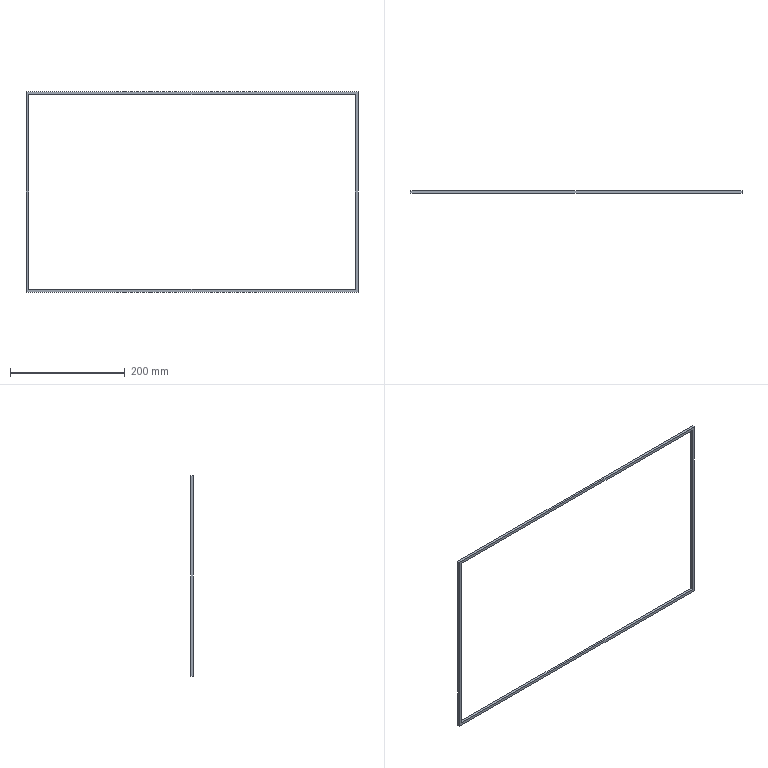Part | SolidWorks | features BaseBody 1 | 1 solid | 10 faces | box 579 x 4.5 x 350 mm | volume 41355 mm3 | plane 10
STEP:
#1=CARTESIAN_POINT('',(-284.5,-3.5,-170.));
#2=VERTEX_POINT('',#1);
#3=CARTESIAN_POINT('',(284.5,-3.5,-170.));
#4=VERTEX_POINT('',#3);
#5=CARTESIAN_POINT('',(0.,-3.5,-170.));
#6=DIRECTION('',(1.,0.,0.));
#7=VECTOR('',#6,1000.);
#8=LINE('',#5,#7);
#9=EDGE_CURVE('',#2,#4,#8,.T.);
#10=ORIENTED_EDGE('',*,*,#9,.F.);
#11=CARTESIAN_POINT('',(-284.5,-3.5,170.));
#12=VERTEX_POINT('',#11);
#13=CARTESIAN_POINT('',(-284.5,-3.5,0.));
#14=DIRECTION('',(0.,0.,-1.));
#15=VECTOR('',#14,1000.);
#16=LINE('',#13,#15);
#17=EDGE_CURVE('',#12,#2,#16,.T.);
#18=ORIENTED_EDGE('',*,*,#17,.F.);
#19=CARTESIAN_POINT('',(284.5,-3.5,170.));
#20=VERTEX_POINT('',#19);
#21=CARTESIAN_POINT('',(0.,-3.5,170.));
#22=DIRECTION('',(-1.,0.,0.));
#23=VECTOR('',#22,1000.);
#24=LINE('',#21,#23);
#25=EDGE_CURVE('',#20,#12,#24,.T.);
#26=ORIENTED_EDGE('',*,*,#25,.F.);
#27=CARTESIAN_POINT('',(284.5,-3.5,0.));
#28=DIRECTION('',(0.,0.,1.));
#29=VECTOR('',#28,1000.);
#30=LINE('',#27,#29);
#31=EDGE_CURVE('',#4,#20,#30,.T.);
#32=ORIENTED_EDGE('',*,*,#31,.F.);
#33=EDGE_LOOP('',(#10,#18,#26,#32));
#34=FACE_BOUND('',#33,.T.);
#35=CARTESIAN_POINT('',(-289.5,-3.5,-175.));
#36=VERTEX_POINT('',#35);
#37=CARTESIAN_POINT('',(-289.5,-3.5,175.));
#38=VERTEX_POINT('',#37);
#39=CARTESIAN_POINT('',(-289.5,-3.5,0.));
#40=DIRECTION('',(0.,0.,1.));
#41=VECTOR('',#40,1000.);
#42=LINE('',#39,#41);
#43=EDGE_CURVE('',#36,#38,#42,.T.);
#44=ORIENTED_EDGE('',*,*,#43,.F.);
#45=CARTESIAN_POINT('',(289.5,-3.5,-175.));
#46=VERTEX_POINT('',#45);
#47=CARTESIAN_POINT('',(0.,-3.5,-175.));
#48=DIRECTION('',(-1.,0.,0.));
#49=VECTOR('',#48,1000.);
#50=LINE('',#47,#49);
#51=EDGE_CURVE('',#46,#36,#50,.T.);
#52=ORIENTED_EDGE('',*,*,#51,.F.);
#53=CARTESIAN_POINT('',(289.5,-3.5,175.));
#54=VERTEX_POINT('',#53);
#55=CARTESIAN_POINT('',(289.5,-3.5,0.));
#56=DIRECTION('',(0.,0.,-1.));
#57=VECTOR('',#56,1000.);
#58=LINE('',#55,#57);
#59=EDGE_CURVE('',#54,#46,#58,.T.);
#60=ORIENTED_EDGE('',*,*,#59,.F.);
#61=CARTESIAN_POINT('',(0.,-3.5,175.));
#62=DIRECTION('',(1.,0.,0.));
#63=VECTOR('',#62,1000.);
#64=LINE('',#61,#63);
#65=EDGE_CURVE('',#38,#54,#64,.T.);
#66=ORIENTED_EDGE('',*,*,#65,.F.);
#67=EDGE_LOOP('',(#44,#52,#60,#66));
#68=FACE_OUTER_BOUND('',#67,.T.);
#69=CARTESIAN_POINT('',(0.,-3.5,0.));
#70=DIRECTION('',(0.,1.,0.));
#71=DIRECTION('',(0.,0.,1.));
#72=AXIS2_PLACEMENT_3D('',#69,#70,#71);
#73=PLANE('',#72);
#74=ADVANCED_FACE('',(#34,#68),#73,.F.);
#75=CARTESIAN_POINT('',(284.5,1.,-170.));
#76=VERTEX_POINT('',#75);
#77=CARTESIAN_POINT('',(284.5,-3.5,-170.));
#78=DIRECTION('',(0.,-1.,0.));
#79=VECTOR('',#78,1000.);
#80=LINE('',#77,#79);
#81=EDGE_CURVE('',#76,#4,#80,.T.);
#82=ORIENTED_EDGE('',*,*,#81,.T.);
#83=ORIENTED_EDGE('',*,*,#31,.T.);
#84=CARTESIAN_POINT('',(284.5,1.,170.));
#85=VERTEX_POINT('',#84);
#86=CARTESIAN_POINT('',(284.5,-3.5,170.));
#87=DIRECTION('',(0.,1.,0.));
#88=VECTOR('',#87,1000.);
#89=LINE('',#86,#88);
#90=EDGE_CURVE('',#20,#85,#89,.T.);
#91=ORIENTED_EDGE('',*,*,#90,.T.);
#92=CARTESIAN_POINT('',(284.5,1.,-170.));
#93=DIRECTION('',(0.,0.,-1.));
#94=VECTOR('',#93,1000.);
#95=LINE('',#92,#94);
#96=EDGE_CURVE('',#85,#76,#95,.T.);
#97=ORIENTED_EDGE('',*,*,#96,.T.);
#98=EDGE_LOOP('',(#82,#83,#91,#97));
#99=FACE_OUTER_BOUND('',#98,.T.);
#100=CARTESIAN_POINT('',(284.5,-3.5,-170.));
#101=DIRECTION('',(-1.,0.,0.));
#102=DIRECTION('',(0.,0.,1.));
#103=AXIS2_PLACEMENT_3D('',#100,#101,#102);
#104=PLANE('',#103);
#105=ADVANCED_FACE('',(#99),#104,.T.);
#106=CARTESIAN_POINT('',(-284.5,1.,-170.));
#107=VERTEX_POINT('',#106);
#108=CARTESIAN_POINT('',(-284.5,-3.5,-170.));
#109=DIRECTION('',(0.,-1.,0.));
#110=VECTOR('',#109,1000.);
#111=LINE('',#108,#110);
#112=EDGE_CURVE('',#107,#2,#111,.T.);
#113=ORIENTED_EDGE('',*,*,#112,.T.);
#114=ORIENTED_EDGE('',*,*,#9,.T.);
#115=ORIENTED_EDGE('',*,*,#81,.F.);
#116=CARTESIAN_POINT('',(-284.5,1.,-170.));
#117=DIRECTION('',(-1.,0.,0.));
#118=VECTOR('',#117,1000.);
#119=LINE('',#116,#118);
#120=EDGE_CURVE('',#76,#107,#119,.T.);
#121=ORIENTED_EDGE('',*,*,#120,.T.);
#122=EDGE_LOOP('',(#113,#114,#115,#121));
#123=FACE_OUTER_BOUND('',#122,.T.);
#124=CARTESIAN_POINT('',(-284.5,-3.5,-170.));
#125=DIRECTION('',(0.,0.,1.));
#126=DIRECTION('',(1.,0.,0.));
#127=AXIS2_PLACEMENT_3D('',#124,#125,#126);
#128=PLANE('',#127);
#129=ADVANCED_FACE('',(#123),#128,.T.);
#130=CARTESIAN_POINT('',(-284.5,1.,170.));
#131=VERTEX_POINT('',#130);
#132=CARTESIAN_POINT('',(-284.5,-3.5,170.));
#133=DIRECTION('',(0.,-1.,0.));
#134=VECTOR('',#133,1000.);
#135=LINE('',#132,#134);
#136=EDGE_CURVE('',#131,#12,#135,.T.);
#137=ORIENTED_EDGE('',*,*,#136,.T.);
#138=ORIENTED_EDGE('',*,*,#17,.T.);
#139=ORIENTED_EDGE('',*,*,#112,.F.);
#140=CARTESIAN_POINT('',(-284.5,1.,170.));
#141=DIRECTION('',(0.,0.,1.));
#142=VECTOR('',#141,1000.);
#143=LINE('',#140,#142);
#144=EDGE_CURVE('',#107,#131,#143,.T.);
#145=ORIENTED_EDGE('',*,*,#144,.T.);
#146=EDGE_LOOP('',(#137,#138,#139,#145));
#147=FACE_OUTER_BOUND('',#146,.T.);
#148=CARTESIAN_POINT('',(-284.5,-3.5,170.));
#149=DIRECTION('',(1.,0.,0.));
#150=DIRECTION('',(0.,0.,-1.));
#151=AXIS2_PLACEMENT_3D('',#148,#149,#150);
#152=PLANE('',#151);
#153=ADVANCED_FACE('',(#147),#152,.T.);
#154=ORIENTED_EDGE('',*,*,#90,.F.);
#155=ORIENTED_EDGE('',*,*,#25,.T.);
#156=ORIENTED_EDGE('',*,*,#136,.F.);
#157=CARTESIAN_POINT('',(284.5,1.,170.));
#158=DIRECTION('',(1.,0.,0.));
#159=VECTOR('',#158,1000.);
#160=LINE('',#157,#159);
#161=EDGE_CURVE('',#131,#85,#160,.T.);
#162=ORIENTED_EDGE('',*,*,#161,.T.);
#163=EDGE_LOOP('',(#154,#155,#156,#162));
#164=FACE_OUTER_BOUND('',#163,.T.);
#165=CARTESIAN_POINT('',(284.5,-3.5,170.));
#166=DIRECTION('',(0.,0.,-1.));
#167=DIRECTION('',(-1.,0.,0.));
#168=AXIS2_PLACEMENT_3D('',#165,#166,#167);
#169=PLANE('',#168);
#170=ADVANCED_FACE('',(#164),#169,.T.);
#171=CARTESIAN_POINT('',(-289.5,1.,175.));
#172=VERTEX_POINT('',#171);
#173=CARTESIAN_POINT('',(-289.5,-3.5,175.));
#174=DIRECTION('',(0.,-1.,0.));
#175=VECTOR('',#174,1000.);
#176=LINE('',#173,#175);
#177=EDGE_CURVE('',#172,#38,#176,.T.);
#178=ORIENTED_EDGE('',*,*,#177,.T.);
#179=ORIENTED_EDGE('',*,*,#65,.T.);
#180=CARTESIAN_POINT('',(289.5,1.,175.));
#181=VERTEX_POINT('',#180);
#182=CARTESIAN_POINT('',(289.5,-3.5,175.));
#183=DIRECTION('',(0.,1.,0.));
#184=VECTOR('',#183,1000.);
#185=LINE('',#182,#184);
#186=EDGE_CURVE('',#54,#181,#185,.T.);
#187=ORIENTED_EDGE('',*,*,#186,.T.);
#188=CARTESIAN_POINT('',(-289.5,1.,175.));
#189=DIRECTION('',(-1.,0.,0.));
#190=VECTOR('',#189,1000.);
#191=LINE('',#188,#190);
#192=EDGE_CURVE('',#181,#172,#191,.T.);
#193=ORIENTED_EDGE('',*,*,#192,.T.);
#194=EDGE_LOOP('',(#178,#179,#187,#193));
#195=FACE_OUTER_BOUND('',#194,.T.);
#196=CARTESIAN_POINT('',(-289.5,-3.5,175.));
#197=DIRECTION('',(0.,0.,1.));
#198=DIRECTION('',(1.,0.,0.));
#199=AXIS2_PLACEMENT_3D('',#196,#197,#198);
#200=PLANE('',#199);
#201=ADVANCED_FACE('',(#195),#200,.T.);
#202=CARTESIAN_POINT('',(-289.5,1.,-175.));
#203=VERTEX_POINT('',#202);
#204=CARTESIAN_POINT('',(-289.5,-3.5,-175.));
#205=DIRECTION('',(0.,-1.,0.));
#206=VECTOR('',#205,1000.);
#207=LINE('',#204,#206);
#208=EDGE_CURVE('',#203,#36,#207,.T.);
#209=ORIENTED_EDGE('',*,*,#208,.T.);
#210=ORIENTED_EDGE('',*,*,#43,.T.);
#211=ORIENTED_EDGE('',*,*,#177,.F.);
#212=CARTESIAN_POINT('',(-289.5,1.,-175.));
#213=DIRECTION('',(0.,0.,-1.));
#214=VECTOR('',#213,1000.);
#215=LINE('',#212,#214);
#216=EDGE_CURVE('',#172,#203,#215,.T.);
#217=ORIENTED_EDGE('',*,*,#216,.T.);
#218=EDGE_LOOP('',(#209,#210,#211,#217));
#219=FACE_OUTER_BOUND('',#218,.T.);
#220=CARTESIAN_POINT('',(-289.5,-3.5,-175.));
#221=DIRECTION('',(-1.,0.,0.));
#222=DIRECTION('',(0.,0.,1.));
#223=AXIS2_PLACEMENT_3D('',#220,#221,#222);
#224=PLANE('',#223);
#225=ADVANCED_FACE('',(#219),#224,.T.);
#226=CARTESIAN_POINT('',(289.5,1.,-175.));
#227=VERTEX_POINT('',#226);
#228=CARTESIAN_POINT('',(289.5,-3.5,-175.));
#229=DIRECTION('',(0.,-1.,0.));
#230=VECTOR('',#229,1000.);
#231=LINE('',#228,#230);
#232=EDGE_CURVE('',#227,#46,#231,.T.);
#233=ORIENTED_EDGE('',*,*,#232,.T.);
#234=ORIENTED_EDGE('',*,*,#51,.T.);
#235=ORIENTED_EDGE('',*,*,#208,.F.);
#236=CARTESIAN_POINT('',(289.5,1.,-175.));
#237=DIRECTION('',(1.,0.,0.));
#238=VECTOR('',#237,1000.);
#239=LINE('',#236,#238);
#240=EDGE_CURVE('',#203,#227,#239,.T.);
#241=ORIENTED_EDGE('',*,*,#240,.T.);
#242=EDGE_LOOP('',(#233,#234,#235,#241));
#243=FACE_OUTER_BOUND('',#242,.T.);
#244=CARTESIAN_POINT('',(289.5,-3.5,-175.));
#245=DIRECTION('',(0.,0.,-1.));
#246=DIRECTION('',(-1.,0.,0.));
#247=AXIS2_PLACEMENT_3D('',#244,#245,#246);
#248=PLANE('',#247);
#249=ADVANCED_FACE('',(#243),#248,.T.);
#250=ORIENTED_EDGE('',*,*,#186,.F.);
#251=ORIENTED_EDGE('',*,*,#59,.T.);
#252=ORIENTED_EDGE('',*,*,#232,.F.);
#253=CARTESIAN_POINT('',(289.5,1.,175.));
#254=DIRECTION('',(0.,0.,1.));
#255=VECTOR('',#254,1000.);
#256=LINE('',#253,#255);
#257=EDGE_CURVE('',#227,#181,#256,.T.);
#258=ORIENTED_EDGE('',*,*,#257,.T.);
#259=EDGE_LOOP('',(#250,#251,#252,#258));
#260=FACE_OUTER_BOUND('',#259,.T.);
#261=CARTESIAN_POINT('',(289.5,-3.5,175.));
#262=DIRECTION('',(1.,0.,0.));
#263=DIRECTION('',(0.,0.,-1.));
#264=AXIS2_PLACEMENT_3D('',#261,#262,#263);
#265=PLANE('',#264);
#266=ADVANCED_FACE('',(#260),#265,.T.);
#267=ORIENTED_EDGE('',*,*,#96,.F.);
#268=ORIENTED_EDGE('',*,*,#161,.F.);
#269=ORIENTED_EDGE('',*,*,#144,.F.);
#270=ORIENTED_EDGE('',*,*,#120,.F.);
#271=EDGE_LOOP('',(#267,#268,#269,#270));
#272=FACE_BOUND('',#271,.T.);
#273=ORIENTED_EDGE('',*,*,#192,.F.);
#274=ORIENTED_EDGE('',*,*,#257,.F.);
#275=ORIENTED_EDGE('',*,*,#240,.F.);
#276=ORIENTED_EDGE('',*,*,#216,.F.);
#277=EDGE_LOOP('',(#273,#274,#275,#276));
#278=FACE_OUTER_BOUND('',#277,.T.);
#279=CARTESIAN_POINT('',(0.,1.,0.));
#280=DIRECTION('',(0.,1.,0.));
#281=DIRECTION('',(0.,0.,1.));
#282=AXIS2_PLACEMENT_3D('',#279,#280,#281);
#283=PLANE('',#282);
#284=ADVANCED_FACE('',(#272,#278),#283,.T.);
#285=CLOSED_SHELL('',(#74,#105,#129,#153,#170,#201,#225,#249,#266,#284));
#286=MANIFOLD_SOLID_BREP('',#285);
#287=CARTESIAN_POINT('',(0.,0.,0.));
#288=DIRECTION('',(0.,0.,1.));
#289=DIRECTION('',(1.,0.,0.));
#290=AXIS2_PLACEMENT_3D('',#287,#288,#289);
#291=(LENGTH_UNIT()NAMED_UNIT(*)SI_UNIT(.MILLI.,.METRE.));
#292=UNCERTAINTY_MEASURE_WITH_UNIT(LENGTH_MEASURE(0.00001),#291,'','');
#293=(NAMED_UNIT(*)PLANE_ANGLE_UNIT()SI_UNIT($,.RADIAN.));
#294=(NAMED_UNIT(*)SI_UNIT($,.STERADIAN.)SOLID_ANGLE_UNIT());
#295=(GEOMETRIC_REPRESENTATION_CONTEXT(3)GLOBAL_UNCERTAINTY_ASSIGNED_CONTEXT((#292))GLOBAL_UNIT_ASSIGNED_CONTEXT((#291,#293,#294))REPRESENTATION_CONTEXT('',''));
#296=ADVANCED_BREP_SHAPE_REPRESENTATION('',(#286,#290),#295);